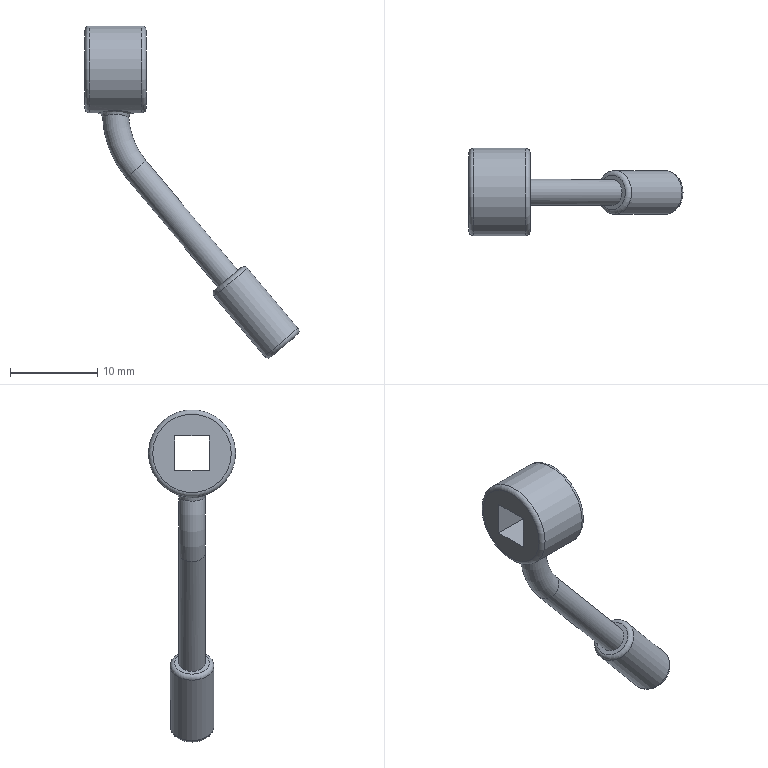Part | STEP file | 1-23.7 | 1 solid | 17 faces | box 24.52 x 10 x 38.054 mm | volume 795.308 mm3 | plane 8 | torus 5 | cylinder 3 | spline 1 | commonest cylinder face diameters 3 x1 5 x1 10 x1